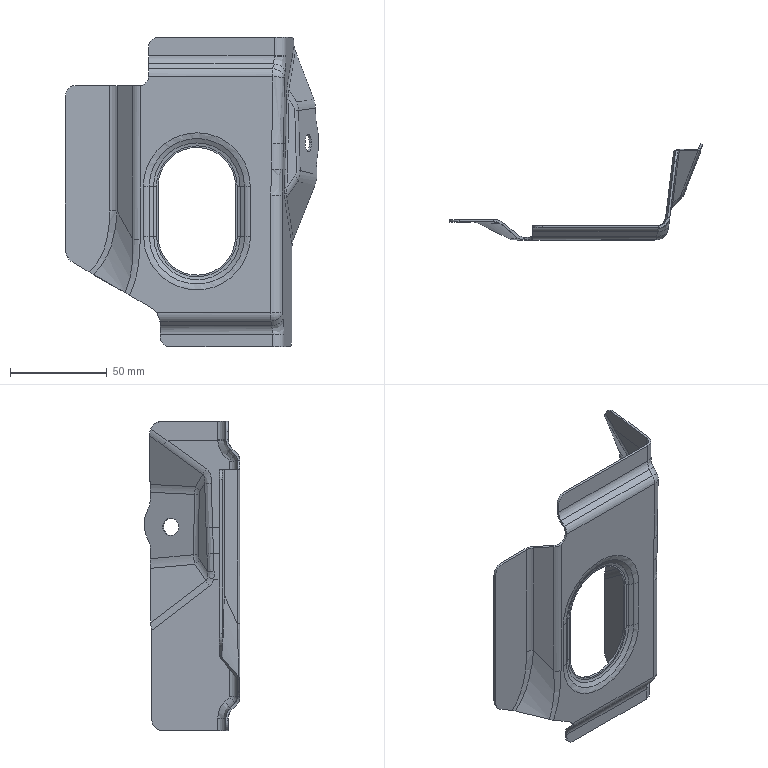Part | STEP file | FNA5401471 | 1 solid | 188 faces | box 130.972 x 49.584 x 160 mm | volume 24899 mm3 | spline 104 | cylinder 52 | plane 21 | other 7 | sphere 4 | commonest cylinder face diameters 12 x13 9.6 x10 10 x3 13.6 x3 14.4 x3 16 x3